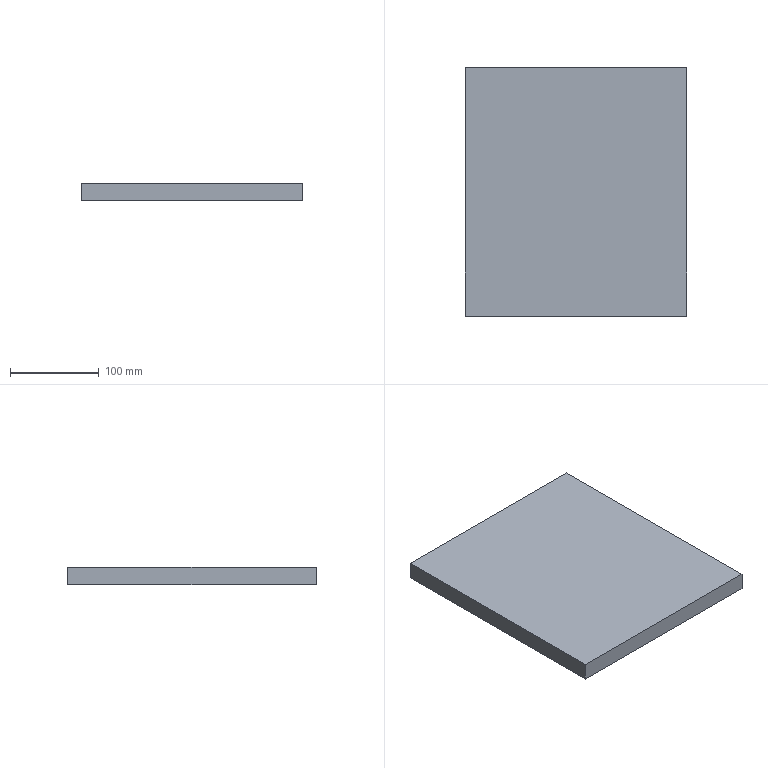Part | SolidWorks | features BaseBody 1 | 1 solid | 6 faces | box 250 x 280 x 20 mm | volume 1400000 mm3 | plane 6
STEP:
#1=CARTESIAN_POINT('',(125.,-140.,0.));
#2=VERTEX_POINT('',#1);
#3=CARTESIAN_POINT('',(125.,140.,0.));
#4=VERTEX_POINT('',#3);
#5=CARTESIAN_POINT('',(125.,140.,0.));
#6=DIRECTION('',(0.,1.,0.));
#7=VECTOR('',#6,1000.);
#8=LINE('',#5,#7);
#9=EDGE_CURVE('',#2,#4,#8,.T.);
#10=ORIENTED_EDGE('',*,*,#9,.F.);
#11=CARTESIAN_POINT('',(-125.,-140.,0.));
#12=VERTEX_POINT('',#11);
#13=CARTESIAN_POINT('',(-125.,-140.,0.));
#14=DIRECTION('',(1.,0.,0.));
#15=VECTOR('',#14,1000.);
#16=LINE('',#13,#15);
#17=EDGE_CURVE('',#12,#2,#16,.T.);
#18=ORIENTED_EDGE('',*,*,#17,.F.);
#19=CARTESIAN_POINT('',(-125.,140.,0.));
#20=VERTEX_POINT('',#19);
#21=CARTESIAN_POINT('',(-125.,140.,0.));
#22=DIRECTION('',(0.,-1.,0.));
#23=VECTOR('',#22,1000.);
#24=LINE('',#21,#23);
#25=EDGE_CURVE('',#20,#12,#24,.T.);
#26=ORIENTED_EDGE('',*,*,#25,.F.);
#27=CARTESIAN_POINT('',(-125.,140.,0.));
#28=DIRECTION('',(-1.,0.,0.));
#29=VECTOR('',#28,1000.);
#30=LINE('',#27,#29);
#31=EDGE_CURVE('',#4,#20,#30,.T.);
#32=ORIENTED_EDGE('',*,*,#31,.F.);
#33=EDGE_LOOP('',(#10,#18,#26,#32));
#34=FACE_OUTER_BOUND('',#33,.T.);
#35=CARTESIAN_POINT('',(0.,0.,0.));
#36=DIRECTION('',(0.,0.,1.));
#37=DIRECTION('',(1.,0.,0.));
#38=AXIS2_PLACEMENT_3D('',#35,#36,#37);
#39=PLANE('',#38);
#40=ADVANCED_FACE('',(#34),#39,.F.);
#41=CARTESIAN_POINT('',(125.,-140.,20.));
#42=VERTEX_POINT('',#41);
#43=CARTESIAN_POINT('',(125.,140.,20.));
#44=VERTEX_POINT('',#43);
#45=CARTESIAN_POINT('',(125.,140.,20.));
#46=DIRECTION('',(0.,1.,0.));
#47=VECTOR('',#46,1000.);
#48=LINE('',#45,#47);
#49=EDGE_CURVE('',#42,#44,#48,.T.);
#50=ORIENTED_EDGE('',*,*,#49,.T.);
#51=CARTESIAN_POINT('',(-125.,140.,20.));
#52=VERTEX_POINT('',#51);
#53=CARTESIAN_POINT('',(-125.,140.,20.));
#54=DIRECTION('',(-1.,0.,0.));
#55=VECTOR('',#54,1000.);
#56=LINE('',#53,#55);
#57=EDGE_CURVE('',#44,#52,#56,.T.);
#58=ORIENTED_EDGE('',*,*,#57,.T.);
#59=CARTESIAN_POINT('',(-125.,-140.,20.));
#60=VERTEX_POINT('',#59);
#61=CARTESIAN_POINT('',(-125.,140.,20.));
#62=DIRECTION('',(0.,-1.,0.));
#63=VECTOR('',#62,1000.);
#64=LINE('',#61,#63);
#65=EDGE_CURVE('',#52,#60,#64,.T.);
#66=ORIENTED_EDGE('',*,*,#65,.T.);
#67=CARTESIAN_POINT('',(-125.,-140.,20.));
#68=DIRECTION('',(1.,0.,0.));
#69=VECTOR('',#68,1000.);
#70=LINE('',#67,#69);
#71=EDGE_CURVE('',#60,#42,#70,.T.);
#72=ORIENTED_EDGE('',*,*,#71,.T.);
#73=EDGE_LOOP('',(#50,#58,#66,#72));
#74=FACE_OUTER_BOUND('',#73,.T.);
#75=CARTESIAN_POINT('',(0.,0.,20.));
#76=DIRECTION('',(0.,0.,1.));
#77=DIRECTION('',(1.,0.,0.));
#78=AXIS2_PLACEMENT_3D('',#75,#76,#77);
#79=PLANE('',#78);
#80=ADVANCED_FACE('',(#74),#79,.T.);
#81=ORIENTED_EDGE('',*,*,#17,.T.);
#82=CARTESIAN_POINT('',(125.,-140.,20.));
#83=DIRECTION('',(0.,0.,-1.));
#84=VECTOR('',#83,1000.);
#85=LINE('',#82,#84);
#86=EDGE_CURVE('',#42,#2,#85,.T.);
#87=ORIENTED_EDGE('',*,*,#86,.F.);
#88=ORIENTED_EDGE('',*,*,#71,.F.);
#89=CARTESIAN_POINT('',(-125.,-140.,20.));
#90=DIRECTION('',(0.,0.,-1.));
#91=VECTOR('',#90,1000.);
#92=LINE('',#89,#91);
#93=EDGE_CURVE('',#60,#12,#92,.T.);
#94=ORIENTED_EDGE('',*,*,#93,.T.);
#95=EDGE_LOOP('',(#81,#87,#88,#94));
#96=FACE_OUTER_BOUND('',#95,.T.);
#97=CARTESIAN_POINT('',(-125.,-140.,20.));
#98=DIRECTION('',(0.,1.,0.));
#99=DIRECTION('',(1.,0.,0.));
#100=AXIS2_PLACEMENT_3D('',#97,#98,#99);
#101=PLANE('',#100);
#102=ADVANCED_FACE('',(#96),#101,.F.);
#103=ORIENTED_EDGE('',*,*,#25,.T.);
#104=ORIENTED_EDGE('',*,*,#93,.F.);
#105=ORIENTED_EDGE('',*,*,#65,.F.);
#106=CARTESIAN_POINT('',(-125.,140.,20.));
#107=DIRECTION('',(0.,0.,-1.));
#108=VECTOR('',#107,1000.);
#109=LINE('',#106,#108);
#110=EDGE_CURVE('',#52,#20,#109,.T.);
#111=ORIENTED_EDGE('',*,*,#110,.T.);
#112=EDGE_LOOP('',(#103,#104,#105,#111));
#113=FACE_OUTER_BOUND('',#112,.T.);
#114=CARTESIAN_POINT('',(-125.,140.,20.));
#115=DIRECTION('',(1.,0.,0.));
#116=DIRECTION('',(0.,1.,0.));
#117=AXIS2_PLACEMENT_3D('',#114,#115,#116);
#118=PLANE('',#117);
#119=ADVANCED_FACE('',(#113),#118,.F.);
#120=ORIENTED_EDGE('',*,*,#31,.T.);
#121=ORIENTED_EDGE('',*,*,#110,.F.);
#122=ORIENTED_EDGE('',*,*,#57,.F.);
#123=CARTESIAN_POINT('',(125.,140.,20.));
#124=DIRECTION('',(0.,0.,-1.));
#125=VECTOR('',#124,1000.);
#126=LINE('',#123,#125);
#127=EDGE_CURVE('',#44,#4,#126,.T.);
#128=ORIENTED_EDGE('',*,*,#127,.T.);
#129=EDGE_LOOP('',(#120,#121,#122,#128));
#130=FACE_OUTER_BOUND('',#129,.T.);
#131=CARTESIAN_POINT('',(-125.,140.,20.));
#132=DIRECTION('',(0.,-1.,0.));
#133=DIRECTION('',(0.,0.,-1.));
#134=AXIS2_PLACEMENT_3D('',#131,#132,#133);
#135=PLANE('',#134);
#136=ADVANCED_FACE('',(#130),#135,.F.);
#137=ORIENTED_EDGE('',*,*,#9,.T.);
#138=ORIENTED_EDGE('',*,*,#127,.F.);
#139=ORIENTED_EDGE('',*,*,#49,.F.);
#140=ORIENTED_EDGE('',*,*,#86,.T.);
#141=EDGE_LOOP('',(#137,#138,#139,#140));
#142=FACE_OUTER_BOUND('',#141,.T.);
#143=CARTESIAN_POINT('',(125.,140.,20.));
#144=DIRECTION('',(-1.,0.,0.));
#145=DIRECTION('',(0.,1.,0.));
#146=AXIS2_PLACEMENT_3D('',#143,#144,#145);
#147=PLANE('',#146);
#148=ADVANCED_FACE('',(#142),#147,.F.);
#149=CLOSED_SHELL('',(#40,#80,#102,#119,#136,#148));
#150=MANIFOLD_SOLID_BREP('',#149);
#151=CARTESIAN_POINT('',(0.,0.,0.));
#152=DIRECTION('',(0.,0.,1.));
#153=DIRECTION('',(1.,0.,0.));
#154=AXIS2_PLACEMENT_3D('',#151,#152,#153);
#155=(LENGTH_UNIT()NAMED_UNIT(*)SI_UNIT(.MILLI.,.METRE.));
#156=UNCERTAINTY_MEASURE_WITH_UNIT(LENGTH_MEASURE(0.00001),#155,'','');
#157=(NAMED_UNIT(*)PLANE_ANGLE_UNIT()SI_UNIT($,.RADIAN.));
#158=(NAMED_UNIT(*)SI_UNIT($,.STERADIAN.)SOLID_ANGLE_UNIT());
#159=(GEOMETRIC_REPRESENTATION_CONTEXT(3)GLOBAL_UNCERTAINTY_ASSIGNED_CONTEXT((#156))GLOBAL_UNIT_ASSIGNED_CONTEXT((#155,#157,#158))REPRESENTATION_CONTEXT('',''));
#160=ADVANCED_BREP_SHAPE_REPRESENTATION('',(#150,#154),#159);